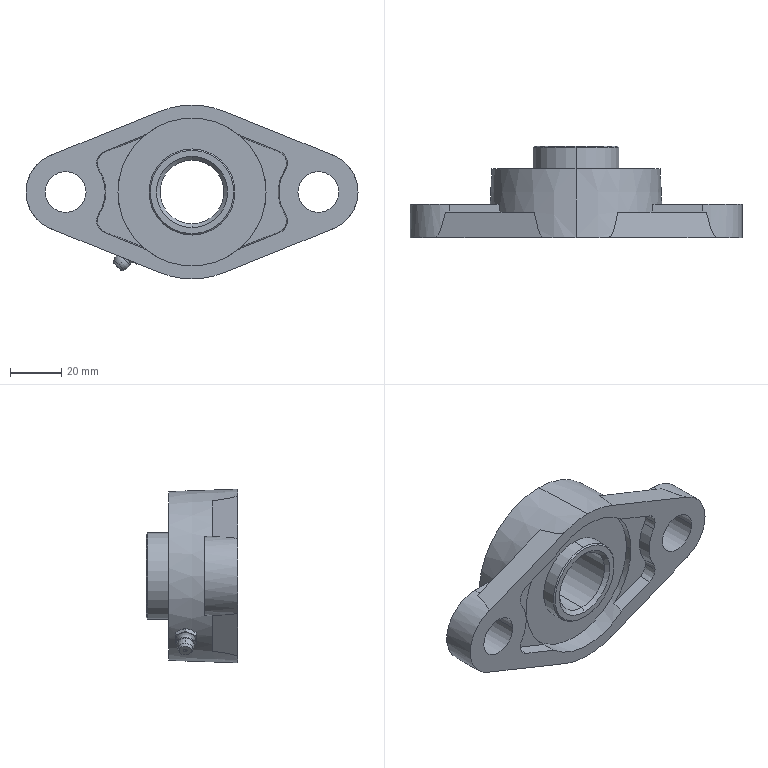Part | STEP file | ucfl2051V11 | 1 solid | 90 faces | box 130 x 35.8 x 68 mm | volume 88119 mm3 | plane 36 | cone 27 | cylinder 19 | torus 4 | sphere 4 | commonest cylinder face diameters 16 x4 33.68 x4 58 x4 31 x3 6 x2 25 x2